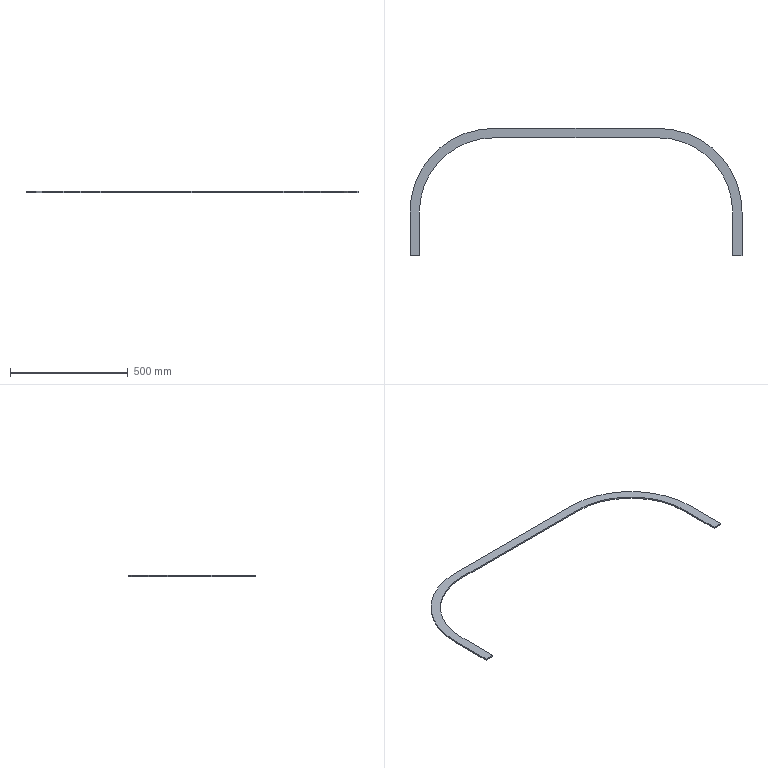Part | NX | features BREP 1 | 1 solid | 14 faces | box 1410 x 540 x 6 mm | volume 509384 mm3 | plane 10 | cylinder 4 | commonest cylinder face diameters 630 x2 710 x2
STEP:
#1=CARTESIAN_POINT('',(0.,315.,0.));
#2=VERTEX_POINT('',#1);
#3=CARTESIAN_POINT('',(315.,0.,0.));
#4=VERTEX_POINT('',#3);
#5=CARTESIAN_POINT('',(0.,0.,0.));
#6=DIRECTION('',(0.,0.,-1.));
#7=DIRECTION('',(1.,0.,0.));
#8=AXIS2_PLACEMENT_3D('',#5,#6,#7);
#9=CIRCLE('',#8,315.);
#10=EDGE_CURVE('',#2,#4,#9,.T.);
#11=ORIENTED_EDGE('',*,*,#10,.T.);
#12=CARTESIAN_POINT('',(315.,0.,6.));
#13=VERTEX_POINT('',#12);
#14=CARTESIAN_POINT('',(315.,0.,6.));
#15=DIRECTION('',(0.,0.,-1.));
#16=VECTOR('',#15,1000.);
#17=LINE('',#14,#16);
#18=EDGE_CURVE('',#13,#4,#17,.T.);
#19=ORIENTED_EDGE('',*,*,#18,.F.);
#20=CARTESIAN_POINT('',(0.,315.,6.));
#21=VERTEX_POINT('',#20);
#22=CARTESIAN_POINT('',(0.,0.,6.));
#23=DIRECTION('',(0.,0.,-1.));
#24=DIRECTION('',(1.,0.,0.));
#25=AXIS2_PLACEMENT_3D('',#22,#23,#24);
#26=CIRCLE('',#25,315.);
#27=EDGE_CURVE('',#21,#13,#26,.T.);
#28=ORIENTED_EDGE('',*,*,#27,.F.);
#29=CARTESIAN_POINT('',(0.,315.,6.));
#30=DIRECTION('',(0.,0.,-1.));
#31=VECTOR('',#30,1000.);
#32=LINE('',#29,#31);
#33=EDGE_CURVE('',#21,#2,#32,.T.);
#34=ORIENTED_EDGE('',*,*,#33,.T.);
#35=EDGE_LOOP('',(#11,#19,#28,#34));
#36=FACE_BOUND('',#35,.T.);
#37=CARTESIAN_POINT('',(0.,0.,6.));
#38=DIRECTION('',(0.,0.,-1.));
#39=DIRECTION('',(1.,0.,0.));
#40=AXIS2_PLACEMENT_3D('',#37,#38,#39);
#41=CYLINDRICAL_SURFACE('',#40,315.);
#42=ADVANCED_FACE('',(#36),#41,.F.);
#43=CARTESIAN_POINT('',(315.,-185.,0.));
#44=VERTEX_POINT('',#43);
#45=CARTESIAN_POINT('',(315.,-185.,0.));
#46=DIRECTION('',(0.,-1.,0.));
#47=VECTOR('',#46,1000.);
#48=LINE('',#45,#47);
#49=EDGE_CURVE('',#4,#44,#48,.T.);
#50=ORIENTED_EDGE('',*,*,#49,.T.);
#51=CARTESIAN_POINT('',(315.,-185.,6.));
#52=VERTEX_POINT('',#51);
#53=CARTESIAN_POINT('',(315.,-185.,6.));
#54=DIRECTION('',(0.,0.,-1.));
#55=VECTOR('',#54,1000.);
#56=LINE('',#53,#55);
#57=EDGE_CURVE('',#52,#44,#56,.T.);
#58=ORIENTED_EDGE('',*,*,#57,.F.);
#59=CARTESIAN_POINT('',(315.,-185.,6.));
#60=DIRECTION('',(0.,-1.,0.));
#61=VECTOR('',#60,1000.);
#62=LINE('',#59,#61);
#63=EDGE_CURVE('',#13,#52,#62,.T.);
#64=ORIENTED_EDGE('',*,*,#63,.F.);
#65=ORIENTED_EDGE('',*,*,#18,.T.);
#66=EDGE_LOOP('',(#50,#58,#64,#65));
#67=FACE_BOUND('',#66,.T.);
#68=CARTESIAN_POINT('',(315.,-185.,6.));
#69=DIRECTION('',(1.,0.,0.));
#70=DIRECTION('',(0.,-1.,0.));
#71=AXIS2_PLACEMENT_3D('',#68,#69,#70);
#72=PLANE('',#71);
#73=ADVANCED_FACE('',(#67),#72,.F.);
#74=CARTESIAN_POINT('',(355.,-185.,0.));
#75=VERTEX_POINT('',#74);
#76=CARTESIAN_POINT('',(315.,-185.,0.));
#77=DIRECTION('',(1.,0.,0.));
#78=VECTOR('',#77,1000.);
#79=LINE('',#76,#78);
#80=EDGE_CURVE('',#44,#75,#79,.T.);
#81=ORIENTED_EDGE('',*,*,#80,.T.);
#82=CARTESIAN_POINT('',(355.,-185.,6.));
#83=VERTEX_POINT('',#82);
#84=CARTESIAN_POINT('',(355.,-185.,6.));
#85=DIRECTION('',(0.,0.,-1.));
#86=VECTOR('',#85,1000.);
#87=LINE('',#84,#86);
#88=EDGE_CURVE('',#83,#75,#87,.T.);
#89=ORIENTED_EDGE('',*,*,#88,.F.);
#90=CARTESIAN_POINT('',(315.,-185.,6.));
#91=DIRECTION('',(1.,0.,0.));
#92=VECTOR('',#91,1000.);
#93=LINE('',#90,#92);
#94=EDGE_CURVE('',#52,#83,#93,.T.);
#95=ORIENTED_EDGE('',*,*,#94,.F.);
#96=ORIENTED_EDGE('',*,*,#57,.T.);
#97=EDGE_LOOP('',(#81,#89,#95,#96));
#98=FACE_BOUND('',#97,.T.);
#99=CARTESIAN_POINT('',(315.,-185.,6.));
#100=DIRECTION('',(0.,1.,0.));
#101=DIRECTION('',(0.,0.,-1.));
#102=AXIS2_PLACEMENT_3D('',#99,#100,#101);
#103=PLANE('',#102);
#104=ADVANCED_FACE('',(#98),#103,.F.);
#105=CARTESIAN_POINT('',(355.,0.,0.));
#106=VERTEX_POINT('',#105);
#107=CARTESIAN_POINT('',(355.,-185.,0.));
#108=DIRECTION('',(0.,1.,0.));
#109=VECTOR('',#108,1000.);
#110=LINE('',#107,#109);
#111=EDGE_CURVE('',#75,#106,#110,.T.);
#112=ORIENTED_EDGE('',*,*,#111,.T.);
#113=CARTESIAN_POINT('',(355.,0.,6.));
#114=VERTEX_POINT('',#113);
#115=CARTESIAN_POINT('',(355.,0.,6.));
#116=DIRECTION('',(0.,0.,-1.));
#117=VECTOR('',#116,1000.);
#118=LINE('',#115,#117);
#119=EDGE_CURVE('',#114,#106,#118,.T.);
#120=ORIENTED_EDGE('',*,*,#119,.F.);
#121=CARTESIAN_POINT('',(355.,-185.,6.));
#122=DIRECTION('',(0.,1.,0.));
#123=VECTOR('',#122,1000.);
#124=LINE('',#121,#123);
#125=EDGE_CURVE('',#83,#114,#124,.T.);
#126=ORIENTED_EDGE('',*,*,#125,.F.);
#127=ORIENTED_EDGE('',*,*,#88,.T.);
#128=EDGE_LOOP('',(#112,#120,#126,#127));
#129=FACE_BOUND('',#128,.T.);
#130=CARTESIAN_POINT('',(355.,-185.,6.));
#131=DIRECTION('',(-1.,0.,0.));
#132=DIRECTION('',(0.,1.,0.));
#133=AXIS2_PLACEMENT_3D('',#130,#131,#132);
#134=PLANE('',#133);
#135=ADVANCED_FACE('',(#129),#134,.F.);
#136=CARTESIAN_POINT('',(0.,355.,0.));
#137=VERTEX_POINT('',#136);
#138=CARTESIAN_POINT('',(0.,0.,0.));
#139=DIRECTION('',(0.,0.,1.));
#140=DIRECTION('',(1.,0.,0.));
#141=AXIS2_PLACEMENT_3D('',#138,#139,#140);
#142=CIRCLE('',#141,355.);
#143=EDGE_CURVE('',#106,#137,#142,.T.);
#144=ORIENTED_EDGE('',*,*,#143,.T.);
#145=CARTESIAN_POINT('',(0.,355.,6.));
#146=VERTEX_POINT('',#145);
#147=CARTESIAN_POINT('',(0.,355.,6.));
#148=DIRECTION('',(0.,0.,-1.));
#149=VECTOR('',#148,1000.);
#150=LINE('',#147,#149);
#151=EDGE_CURVE('',#146,#137,#150,.T.);
#152=ORIENTED_EDGE('',*,*,#151,.F.);
#153=CARTESIAN_POINT('',(0.,0.,6.));
#154=DIRECTION('',(0.,0.,1.));
#155=DIRECTION('',(1.,0.,0.));
#156=AXIS2_PLACEMENT_3D('',#153,#154,#155);
#157=CIRCLE('',#156,355.);
#158=EDGE_CURVE('',#114,#146,#157,.T.);
#159=ORIENTED_EDGE('',*,*,#158,.F.);
#160=ORIENTED_EDGE('',*,*,#119,.T.);
#161=EDGE_LOOP('',(#144,#152,#159,#160));
#162=FACE_BOUND('',#161,.T.);
#163=CARTESIAN_POINT('',(0.,0.,6.));
#164=DIRECTION('',(0.,0.,-1.));
#165=DIRECTION('',(1.,0.,0.));
#166=AXIS2_PLACEMENT_3D('',#163,#164,#165);
#167=CYLINDRICAL_SURFACE('',#166,355.);
#168=ADVANCED_FACE('',(#162),#167,.T.);
#169=CARTESIAN_POINT('',(-700.,355.,0.));
#170=VERTEX_POINT('',#169);
#171=CARTESIAN_POINT('',(0.,355.,0.));
#172=DIRECTION('',(-1.,0.,0.));
#173=VECTOR('',#172,1000.);
#174=LINE('',#171,#173);
#175=EDGE_CURVE('',#137,#170,#174,.T.);
#176=ORIENTED_EDGE('',*,*,#175,.T.);
#177=CARTESIAN_POINT('',(-700.,355.,6.));
#178=VERTEX_POINT('',#177);
#179=CARTESIAN_POINT('',(-700.,355.,6.));
#180=DIRECTION('',(0.,0.,-1.));
#181=VECTOR('',#180,1000.);
#182=LINE('',#179,#181);
#183=EDGE_CURVE('',#178,#170,#182,.T.);
#184=ORIENTED_EDGE('',*,*,#183,.F.);
#185=CARTESIAN_POINT('',(0.,355.,6.));
#186=DIRECTION('',(-1.,0.,0.));
#187=VECTOR('',#186,1000.);
#188=LINE('',#185,#187);
#189=EDGE_CURVE('',#146,#178,#188,.T.);
#190=ORIENTED_EDGE('',*,*,#189,.F.);
#191=ORIENTED_EDGE('',*,*,#151,.T.);
#192=EDGE_LOOP('',(#176,#184,#190,#191));
#193=FACE_BOUND('',#192,.T.);
#194=CARTESIAN_POINT('',(0.,355.,6.));
#195=DIRECTION('',(0.,-1.,0.));
#196=DIRECTION('',(0.,0.,1.));
#197=AXIS2_PLACEMENT_3D('',#194,#195,#196);
#198=PLANE('',#197);
#199=ADVANCED_FACE('',(#193),#198,.F.);
#200=CARTESIAN_POINT('',(-1055.,0.,0.));
#201=VERTEX_POINT('',#200);
#202=CARTESIAN_POINT('',(-700.,0.,0.));
#203=DIRECTION('',(0.,0.,1.));
#204=DIRECTION('',(1.,0.,0.));
#205=AXIS2_PLACEMENT_3D('',#202,#203,#204);
#206=CIRCLE('',#205,355.);
#207=EDGE_CURVE('',#170,#201,#206,.T.);
#208=ORIENTED_EDGE('',*,*,#207,.T.);
#209=CARTESIAN_POINT('',(-1055.,0.,6.));
#210=VERTEX_POINT('',#209);
#211=CARTESIAN_POINT('',(-1055.,0.,6.));
#212=DIRECTION('',(0.,0.,-1.));
#213=VECTOR('',#212,1000.);
#214=LINE('',#211,#213);
#215=EDGE_CURVE('',#210,#201,#214,.T.);
#216=ORIENTED_EDGE('',*,*,#215,.F.);
#217=CARTESIAN_POINT('',(-700.,0.,6.));
#218=DIRECTION('',(0.,0.,1.));
#219=DIRECTION('',(1.,0.,0.));
#220=AXIS2_PLACEMENT_3D('',#217,#218,#219);
#221=CIRCLE('',#220,355.);
#222=EDGE_CURVE('',#178,#210,#221,.T.);
#223=ORIENTED_EDGE('',*,*,#222,.F.);
#224=ORIENTED_EDGE('',*,*,#183,.T.);
#225=EDGE_LOOP('',(#208,#216,#223,#224));
#226=FACE_BOUND('',#225,.T.);
#227=CARTESIAN_POINT('',(-700.,0.,6.));
#228=DIRECTION('',(0.,0.,-1.));
#229=DIRECTION('',(1.,0.,0.));
#230=AXIS2_PLACEMENT_3D('',#227,#228,#229);
#231=CYLINDRICAL_SURFACE('',#230,355.);
#232=ADVANCED_FACE('',(#226),#231,.T.);
#233=CARTESIAN_POINT('',(-1055.,-185.,0.));
#234=VERTEX_POINT('',#233);
#235=CARTESIAN_POINT('',(-1055.,0.,0.));
#236=DIRECTION('',(0.,-1.,0.));
#237=VECTOR('',#236,1000.);
#238=LINE('',#235,#237);
#239=EDGE_CURVE('',#201,#234,#238,.T.);
#240=ORIENTED_EDGE('',*,*,#239,.T.);
#241=CARTESIAN_POINT('',(-1055.,-185.,6.));
#242=VERTEX_POINT('',#241);
#243=CARTESIAN_POINT('',(-1055.,-185.,6.));
#244=DIRECTION('',(0.,0.,-1.));
#245=VECTOR('',#244,1000.);
#246=LINE('',#243,#245);
#247=EDGE_CURVE('',#242,#234,#246,.T.);
#248=ORIENTED_EDGE('',*,*,#247,.F.);
#249=CARTESIAN_POINT('',(-1055.,0.,6.));
#250=DIRECTION('',(0.,-1.,0.));
#251=VECTOR('',#250,1000.);
#252=LINE('',#249,#251);
#253=EDGE_CURVE('',#210,#242,#252,.T.);
#254=ORIENTED_EDGE('',*,*,#253,.F.);
#255=ORIENTED_EDGE('',*,*,#215,.T.);
#256=EDGE_LOOP('',(#240,#248,#254,#255));
#257=FACE_BOUND('',#256,.T.);
#258=CARTESIAN_POINT('',(-1055.,0.,6.));
#259=DIRECTION('',(1.,0.,0.));
#260=DIRECTION('',(0.,-1.,0.));
#261=AXIS2_PLACEMENT_3D('',#258,#259,#260);
#262=PLANE('',#261);
#263=ADVANCED_FACE('',(#257),#262,.F.);
#264=CARTESIAN_POINT('',(-1015.,-185.,0.));
#265=VERTEX_POINT('',#264);
#266=CARTESIAN_POINT('',(-1055.,-185.,0.));
#267=DIRECTION('',(1.,0.,0.));
#268=VECTOR('',#267,1000.);
#269=LINE('',#266,#268);
#270=EDGE_CURVE('',#234,#265,#269,.T.);
#271=ORIENTED_EDGE('',*,*,#270,.T.);
#272=CARTESIAN_POINT('',(-1015.,-185.,6.));
#273=VERTEX_POINT('',#272);
#274=CARTESIAN_POINT('',(-1015.,-185.,6.));
#275=DIRECTION('',(0.,0.,-1.));
#276=VECTOR('',#275,1000.);
#277=LINE('',#274,#276);
#278=EDGE_CURVE('',#273,#265,#277,.T.);
#279=ORIENTED_EDGE('',*,*,#278,.F.);
#280=CARTESIAN_POINT('',(-1055.,-185.,6.));
#281=DIRECTION('',(1.,0.,0.));
#282=VECTOR('',#281,1000.);
#283=LINE('',#280,#282);
#284=EDGE_CURVE('',#242,#273,#283,.T.);
#285=ORIENTED_EDGE('',*,*,#284,.F.);
#286=ORIENTED_EDGE('',*,*,#247,.T.);
#287=EDGE_LOOP('',(#271,#279,#285,#286));
#288=FACE_BOUND('',#287,.T.);
#289=CARTESIAN_POINT('',(-1055.,-185.,6.));
#290=DIRECTION('',(0.,1.,0.));
#291=DIRECTION('',(0.,0.,-1.));
#292=AXIS2_PLACEMENT_3D('',#289,#290,#291);
#293=PLANE('',#292);
#294=ADVANCED_FACE('',(#288),#293,.F.);
#295=CARTESIAN_POINT('',(-1015.,0.,0.));
#296=VERTEX_POINT('',#295);
#297=CARTESIAN_POINT('',(-1015.,0.,0.));
#298=DIRECTION('',(0.,1.,0.));
#299=VECTOR('',#298,1000.);
#300=LINE('',#297,#299);
#301=EDGE_CURVE('',#265,#296,#300,.T.);
#302=ORIENTED_EDGE('',*,*,#301,.T.);
#303=CARTESIAN_POINT('',(-1015.,0.,6.));
#304=VERTEX_POINT('',#303);
#305=CARTESIAN_POINT('',(-1015.,0.,6.));
#306=DIRECTION('',(0.,0.,-1.));
#307=VECTOR('',#306,1000.);
#308=LINE('',#305,#307);
#309=EDGE_CURVE('',#304,#296,#308,.T.);
#310=ORIENTED_EDGE('',*,*,#309,.F.);
#311=CARTESIAN_POINT('',(-1015.,0.,6.));
#312=DIRECTION('',(0.,1.,0.));
#313=VECTOR('',#312,1000.);
#314=LINE('',#311,#313);
#315=EDGE_CURVE('',#273,#304,#314,.T.);
#316=ORIENTED_EDGE('',*,*,#315,.F.);
#317=ORIENTED_EDGE('',*,*,#278,.T.);
#318=EDGE_LOOP('',(#302,#310,#316,#317));
#319=FACE_BOUND('',#318,.T.);
#320=CARTESIAN_POINT('',(-1015.,0.,6.));
#321=DIRECTION('',(-1.,0.,0.));
#322=DIRECTION('',(0.,0.,-1.));
#323=AXIS2_PLACEMENT_3D('',#320,#321,#322);
#324=PLANE('',#323);
#325=ADVANCED_FACE('',(#319),#324,.F.);
#326=CARTESIAN_POINT('',(-700.,315.,0.));
#327=VERTEX_POINT('',#326);
#328=CARTESIAN_POINT('',(-700.,0.,0.));
#329=DIRECTION('',(0.,0.,-1.));
#330=DIRECTION('',(1.,0.,0.));
#331=AXIS2_PLACEMENT_3D('',#328,#329,#330);
#332=CIRCLE('',#331,315.);
#333=EDGE_CURVE('',#296,#327,#332,.T.);
#334=ORIENTED_EDGE('',*,*,#333,.T.);
#335=CARTESIAN_POINT('',(-700.,315.,6.));
#336=VERTEX_POINT('',#335);
#337=CARTESIAN_POINT('',(-700.,315.,6.));
#338=DIRECTION('',(0.,0.,-1.));
#339=VECTOR('',#338,1000.);
#340=LINE('',#337,#339);
#341=EDGE_CURVE('',#336,#327,#340,.T.);
#342=ORIENTED_EDGE('',*,*,#341,.F.);
#343=CARTESIAN_POINT('',(-700.,0.,6.));
#344=DIRECTION('',(0.,0.,-1.));
#345=DIRECTION('',(1.,0.,0.));
#346=AXIS2_PLACEMENT_3D('',#343,#344,#345);
#347=CIRCLE('',#346,315.);
#348=EDGE_CURVE('',#304,#336,#347,.T.);
#349=ORIENTED_EDGE('',*,*,#348,.F.);
#350=ORIENTED_EDGE('',*,*,#309,.T.);
#351=EDGE_LOOP('',(#334,#342,#349,#350));
#352=FACE_BOUND('',#351,.T.);
#353=CARTESIAN_POINT('',(-700.,0.,6.));
#354=DIRECTION('',(0.,0.,-1.));
#355=DIRECTION('',(1.,0.,0.));
#356=AXIS2_PLACEMENT_3D('',#353,#354,#355);
#357=CYLINDRICAL_SURFACE('',#356,315.);
#358=ADVANCED_FACE('',(#352),#357,.F.);
#359=CARTESIAN_POINT('',(0.,315.,0.));
#360=DIRECTION('',(1.,0.,0.));
#361=VECTOR('',#360,1000.);
#362=LINE('',#359,#361);
#363=EDGE_CURVE('',#327,#2,#362,.T.);
#364=ORIENTED_EDGE('',*,*,#363,.T.);
#365=ORIENTED_EDGE('',*,*,#33,.F.);
#366=CARTESIAN_POINT('',(0.,315.,6.));
#367=DIRECTION('',(1.,0.,0.));
#368=VECTOR('',#367,1000.);
#369=LINE('',#366,#368);
#370=EDGE_CURVE('',#336,#21,#369,.T.);
#371=ORIENTED_EDGE('',*,*,#370,.F.);
#372=ORIENTED_EDGE('',*,*,#341,.T.);
#373=EDGE_LOOP('',(#364,#365,#371,#372));
#374=FACE_BOUND('',#373,.T.);
#375=CARTESIAN_POINT('',(0.,315.,6.));
#376=DIRECTION('',(0.,1.,0.));
#377=DIRECTION('',(0.,0.,-1.));
#378=AXIS2_PLACEMENT_3D('',#375,#376,#377);
#379=PLANE('',#378);
#380=ADVANCED_FACE('',(#374),#379,.F.);
#381=ORIENTED_EDGE('',*,*,#27,.T.);
#382=ORIENTED_EDGE('',*,*,#63,.T.);
#383=ORIENTED_EDGE('',*,*,#94,.T.);
#384=ORIENTED_EDGE('',*,*,#125,.T.);
#385=ORIENTED_EDGE('',*,*,#158,.T.);
#386=ORIENTED_EDGE('',*,*,#189,.T.);
#387=ORIENTED_EDGE('',*,*,#222,.T.);
#388=ORIENTED_EDGE('',*,*,#253,.T.);
#389=ORIENTED_EDGE('',*,*,#284,.T.);
#390=ORIENTED_EDGE('',*,*,#315,.T.);
#391=ORIENTED_EDGE('',*,*,#348,.T.);
#392=ORIENTED_EDGE('',*,*,#370,.T.);
#393=EDGE_LOOP('',(#381,#382,#383,#384,#385,#386,#387,#388,#389,#390,#391,#392));
#394=FACE_BOUND('',#393,.T.);
#395=CARTESIAN_POINT('',(0.,0.,6.));
#396=DIRECTION('',(0.,0.,1.));
#397=DIRECTION('',(-1.,0.,0.));
#398=AXIS2_PLACEMENT_3D('',#395,#396,#397);
#399=PLANE('',#398);
#400=ADVANCED_FACE('',(#394),#399,.T.);
#401=ORIENTED_EDGE('',*,*,#10,.F.);
#402=ORIENTED_EDGE('',*,*,#363,.F.);
#403=ORIENTED_EDGE('',*,*,#333,.F.);
#404=ORIENTED_EDGE('',*,*,#301,.F.);
#405=ORIENTED_EDGE('',*,*,#270,.F.);
#406=ORIENTED_EDGE('',*,*,#239,.F.);
#407=ORIENTED_EDGE('',*,*,#207,.F.);
#408=ORIENTED_EDGE('',*,*,#175,.F.);
#409=ORIENTED_EDGE('',*,*,#143,.F.);
#410=ORIENTED_EDGE('',*,*,#111,.F.);
#411=ORIENTED_EDGE('',*,*,#80,.F.);
#412=ORIENTED_EDGE('',*,*,#49,.F.);
#413=EDGE_LOOP('',(#401,#402,#403,#404,#405,#406,#407,#408,#409,#410,#411,#412));
#414=FACE_BOUND('',#413,.T.);
#415=CARTESIAN_POINT('',(0.,0.,0.));
#416=DIRECTION('',(0.,0.,1.));
#417=DIRECTION('',(-1.,0.,0.));
#418=AXIS2_PLACEMENT_3D('',#415,#416,#417);
#419=PLANE('',#418);
#420=ADVANCED_FACE('',(#414),#419,.F.);
#421=CLOSED_SHELL('',(#42,#73,#104,#135,#168,#199,#232,#263,#294,#325,#358,#380,#400,#420));
#422=MANIFOLD_SOLID_BREP('',#421);
#423=(LENGTH_UNIT()NAMED_UNIT(*)SI_UNIT(.MILLI.,.METRE.));
#424=UNCERTAINTY_MEASURE_WITH_UNIT(LENGTH_MEASURE(0.00001),#423,'','');
#425=(NAMED_UNIT(*)PLANE_ANGLE_UNIT()SI_UNIT($,.RADIAN.));
#426=(NAMED_UNIT(*)SI_UNIT($,.STERADIAN.)SOLID_ANGLE_UNIT());
#427=(GEOMETRIC_REPRESENTATION_CONTEXT(3)GLOBAL_UNCERTAINTY_ASSIGNED_CONTEXT((#424))GLOBAL_UNIT_ASSIGNED_CONTEXT((#423,#425,#426))REPRESENTATION_CONTEXT('',''));
#428=ADVANCED_BREP_SHAPE_REPRESENTATION('',(#422),#427);